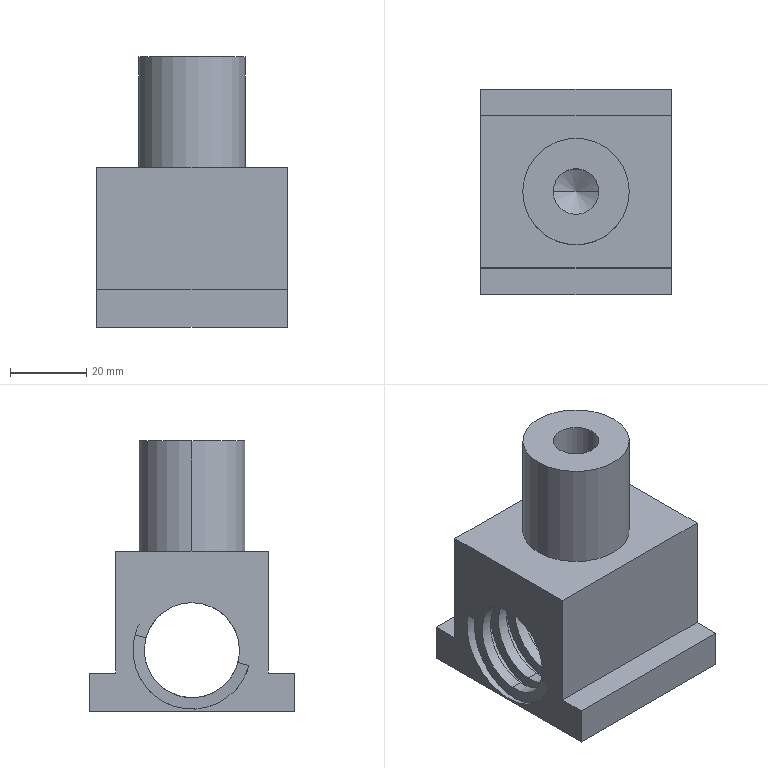Part | SolidWorks | features ICE 3, Extrusion 1, Helix 1, RevCut 1, SweepCut 1 | 1 solid | 39 faces | box 50 x 54 x 71 mm | volume 75271 mm3 | cylinder 23 | plane 11 | spline 3 | cone 2 | commonest cylinder face diameters 25 x19 12 x2 28 x2